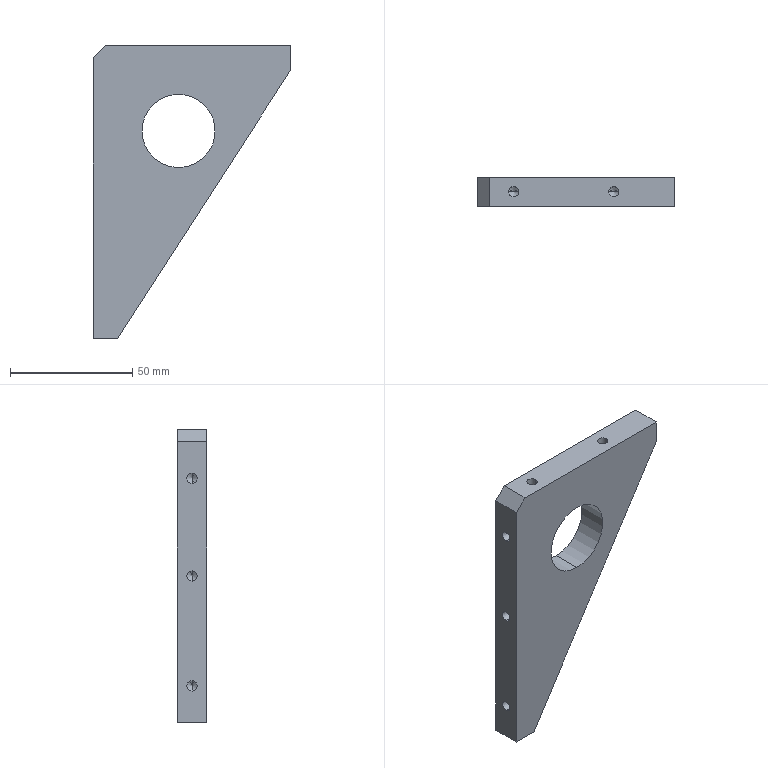Part | STEP file | PN_0015 | 1 solid | 30 faces | box 81 x 12 x 120 mm | volume 60149 mm3 | cylinder 12 | cone 10 | plane 8 | commonest cylinder face diameters 4.2 x10 30 x2